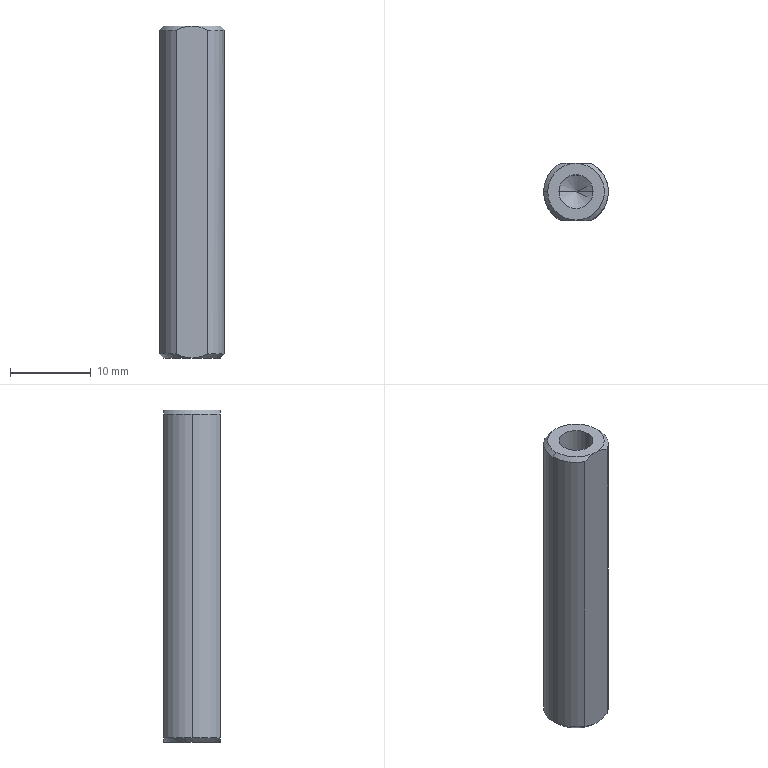Part | STEP file | 11-FG-B08411 | 1 solid | 17 faces | box 8 x 7 x 41 mm | volume 1772 mm3 | cone 8 | cylinder 5 | plane 4 | commonest cylinder face diameters 8 x3 4.2 x2
STEP:
#1=CARTESIAN_POINT('',(3.5,0.,0.));
#2=VERTEX_POINT('',#1);
#3=CARTESIAN_POINT('',(0.,-3.5,0.));
#4=VERTEX_POINT('',#3);
#5=CARTESIAN_POINT('',(0.,0.,0.));
#6=DIRECTION('',(0.,0.,-1.));
#7=DIRECTION('',(1.,0.,0.));
#8=AXIS2_PLACEMENT_3D('',#5,#6,#7);
#9=CIRCLE('',#8,3.5);
#10=EDGE_CURVE('',#2,#4,#9,.T.);
#11=ORIENTED_EDGE('',*,*,#10,.F.);
#12=CARTESIAN_POINT('',(4.,0.,0.5));
#13=VERTEX_POINT('',#12);
#14=CARTESIAN_POINT('',(4.,0.,0.5));
#15=DIRECTION('',(0.7071,0.,0.7071));
#16=VECTOR('',#15,1000.);
#17=LINE('',#14,#16);
#18=EDGE_CURVE('',#2,#13,#17,.T.);
#19=ORIENTED_EDGE('',*,*,#18,.T.);
#20=CARTESIAN_POINT('',(1.936,-3.5,0.5));
#21=VERTEX_POINT('',#20);
#22=CARTESIAN_POINT('',(0.,0.,0.5));
#23=DIRECTION('',(0.,0.,1.));
#24=DIRECTION('',(1.,0.,0.));
#25=AXIS2_PLACEMENT_3D('',#22,#23,#24);
#26=CIRCLE('',#25,4.);
#27=EDGE_CURVE('',#21,#13,#26,.T.);
#28=ORIENTED_EDGE('',*,*,#27,.F.);
#29=CARTESIAN_POINT('',(0.,-3.5,0.));
#30=CARTESIAN_POINT('',(0.3398,-3.5,0.));
#31=CARTESIAN_POINT('',(0.6708,-3.5,0.05004));
#32=CARTESIAN_POINT('',(1.157,-3.5,0.183));
#33=CARTESIAN_POINT('',(1.318,-3.5,0.2372));
#34=CARTESIAN_POINT('',(1.633,-3.5,0.3594));
#35=CARTESIAN_POINT('',(1.786,-3.5,0.4272));
#36=CARTESIAN_POINT('',(1.936,-3.5,0.5));
#37=B_SPLINE_CURVE_WITH_KNOTS('',3,(#29,#30,#31,#32,#33,#34,#35,#36),.UNSPECIFIED.,.F.,.F.,(4,2,2,4),(0.004539,0.00554,0.00604,0.006541),.UNSPECIFIED.);
#38=EDGE_CURVE('',#4,#21,#37,.T.);
#39=ORIENTED_EDGE('',*,*,#38,.F.);
#40=EDGE_LOOP('',(#11,#19,#28,#39));
#41=FACE_OUTER_BOUND('',#40,.T.);
#42=CARTESIAN_POINT('',(0.,0.,0.5));
#43=DIRECTION('',(0.,0.,1.));
#44=DIRECTION('',(1.,0.,0.));
#45=AXIS2_PLACEMENT_3D('',#42,#43,#44);
#46=CONICAL_SURFACE('',#45,4.,0.7854);
#47=ADVANCED_FACE('',(#41),#46,.T.);
#48=CARTESIAN_POINT('',(-3.5,0.,41.));
#49=VERTEX_POINT('',#48);
#50=CARTESIAN_POINT('',(0.,-3.5,41.));
#51=VERTEX_POINT('',#50);
#52=CARTESIAN_POINT('',(0.,0.,41.));
#53=DIRECTION('',(0.,0.,1.));
#54=DIRECTION('',(1.,0.,0.));
#55=AXIS2_PLACEMENT_3D('',#52,#53,#54);
#56=CIRCLE('',#55,3.5);
#57=EDGE_CURVE('',#49,#51,#56,.T.);
#58=ORIENTED_EDGE('',*,*,#57,.F.);
#59=CARTESIAN_POINT('',(-4.,0.,40.5));
#60=VERTEX_POINT('',#59);
#61=CARTESIAN_POINT('',(-3.5,0.,41.));
#62=DIRECTION('',(-0.7071,0.,-0.7071));
#63=VECTOR('',#62,1000.);
#64=LINE('',#61,#63);
#65=EDGE_CURVE('',#49,#60,#64,.T.);
#66=ORIENTED_EDGE('',*,*,#65,.T.);
#67=CARTESIAN_POINT('',(-1.936,-3.5,40.5));
#68=VERTEX_POINT('',#67);
#69=CARTESIAN_POINT('',(0.,0.,40.5));
#70=DIRECTION('',(0.,0.,-1.));
#71=DIRECTION('',(1.,0.,0.));
#72=AXIS2_PLACEMENT_3D('',#69,#70,#71);
#73=CIRCLE('',#72,4.);
#74=EDGE_CURVE('',#68,#60,#73,.T.);
#75=ORIENTED_EDGE('',*,*,#74,.F.);
#76=CARTESIAN_POINT('',(0.,-3.5,41.));
#77=CARTESIAN_POINT('',(-0.3397,-3.5,41.));
#78=CARTESIAN_POINT('',(-0.6719,-3.5,40.95));
#79=CARTESIAN_POINT('',(-1.318,-3.5,40.773));
#80=CARTESIAN_POINT('',(-1.635,-3.5,40.646));
#81=CARTESIAN_POINT('',(-1.936,-3.5,40.5));
#82=B_SPLINE_CURVE_WITH_KNOTS('',3,(#76,#77,#78,#79,#80,#81),.UNSPECIFIED.,.F.,.F.,(4,2,4),(0.004275,0.005275,0.006275),.UNSPECIFIED.);
#83=EDGE_CURVE('',#51,#68,#82,.T.);
#84=ORIENTED_EDGE('',*,*,#83,.F.);
#85=EDGE_LOOP('',(#58,#66,#75,#84));
#86=FACE_OUTER_BOUND('',#85,.T.);
#87=CARTESIAN_POINT('',(0.,0.,41.));
#88=DIRECTION('',(0.,0.,-1.));
#89=DIRECTION('',(-1.,0.,0.));
#90=AXIS2_PLACEMENT_3D('',#87,#88,#89);
#91=CONICAL_SURFACE('',#90,3.5,0.7854);
#92=ADVANCED_FACE('',(#86),#91,.T.);
#93=CARTESIAN_POINT('',(-2.1,0.,28.6));
#94=VERTEX_POINT('',#93);
#95=CARTESIAN_POINT('',(2.1,0.,28.6));
#96=VERTEX_POINT('',#95);
#97=CARTESIAN_POINT('',(0.,0.,28.6));
#98=DIRECTION('',(0.,0.,1.));
#99=DIRECTION('',(1.,0.,0.));
#100=AXIS2_PLACEMENT_3D('',#97,#98,#99);
#101=CIRCLE('',#100,2.1);
#102=EDGE_CURVE('',#94,#96,#101,.T.);
#103=ORIENTED_EDGE('',*,*,#102,.F.);
#104=CARTESIAN_POINT('',(-2.1,0.,41.));
#105=VERTEX_POINT('',#104);
#106=CARTESIAN_POINT('',(-2.1,0.,41.));
#107=DIRECTION('',(0.,0.,1.));
#108=VECTOR('',#107,1000.);
#109=LINE('',#106,#108);
#110=EDGE_CURVE('',#94,#105,#109,.T.);
#111=ORIENTED_EDGE('',*,*,#110,.T.);
#112=CARTESIAN_POINT('',(2.1,0.,41.));
#113=VERTEX_POINT('',#112);
#114=CARTESIAN_POINT('',(0.,0.,41.));
#115=DIRECTION('',(0.,0.,1.));
#116=DIRECTION('',(1.,0.,0.));
#117=AXIS2_PLACEMENT_3D('',#114,#115,#116);
#118=CIRCLE('',#117,2.1);
#119=EDGE_CURVE('',#105,#113,#118,.T.);
#120=ORIENTED_EDGE('',*,*,#119,.T.);
#121=CARTESIAN_POINT('',(2.1,0.,41.));
#122=DIRECTION('',(0.,0.,1.));
#123=VECTOR('',#122,1000.);
#124=LINE('',#121,#123);
#125=EDGE_CURVE('',#96,#113,#124,.T.);
#126=ORIENTED_EDGE('',*,*,#125,.F.);
#127=EDGE_LOOP('',(#103,#111,#120,#126));
#128=FACE_OUTER_BOUND('',#127,.T.);
#129=CARTESIAN_POINT('',(0.,0.,41.));
#130=DIRECTION('',(0.,0.,1.));
#131=DIRECTION('',(1.,0.,0.));
#132=AXIS2_PLACEMENT_3D('',#129,#130,#131);
#133=CYLINDRICAL_SURFACE('',#132,2.1);
#134=ADVANCED_FACE('',(#128),#133,.F.);
#135=CARTESIAN_POINT('',(0.,0.,27.338));
#136=VERTEX_POINT('',#135);
#137=CARTESIAN_POINT('',(2.1,0.,28.6));
#138=DIRECTION('',(0.8572,0.,0.515));
#139=VECTOR('',#138,1000.);
#140=LINE('',#137,#139);
#141=EDGE_CURVE('',#136,#96,#140,.T.);
#142=ORIENTED_EDGE('',*,*,#141,.F.);
#143=CARTESIAN_POINT('',(-2.1,0.,28.6));
#144=DIRECTION('',(-0.8572,0.,0.515));
#145=VECTOR('',#144,1000.);
#146=LINE('',#143,#145);
#147=EDGE_CURVE('',#136,#94,#146,.T.);
#148=ORIENTED_EDGE('',*,*,#147,.T.);
#149=ORIENTED_EDGE('',*,*,#102,.T.);
#150=EDGE_LOOP('',(#142,#148,#149));
#151=FACE_OUTER_BOUND('',#150,.T.);
#152=CARTESIAN_POINT('',(0.,0.,28.6));
#153=DIRECTION('',(0.,0.,1.));
#154=DIRECTION('',(1.,0.,0.));
#155=AXIS2_PLACEMENT_3D('',#152,#153,#154);
#156=CONICAL_SURFACE('',#155,2.1,1.03);
#157=ADVANCED_FACE('',(#151),#156,.F.);
#158=ORIENTED_EDGE('',*,*,#74,.T.);
#159=CARTESIAN_POINT('',(-4.,0.,0.5));
#160=VERTEX_POINT('',#159);
#161=CARTESIAN_POINT('',(-4.,0.,41.));
#162=DIRECTION('',(0.,0.,-1.));
#163=VECTOR('',#162,1000.);
#164=LINE('',#161,#163);
#165=EDGE_CURVE('',#60,#160,#164,.T.);
#166=ORIENTED_EDGE('',*,*,#165,.T.);
#167=CARTESIAN_POINT('',(-1.936,-3.5,0.5));
#168=VERTEX_POINT('',#167);
#169=CARTESIAN_POINT('',(0.,0.,0.5));
#170=DIRECTION('',(0.,0.,1.));
#171=DIRECTION('',(1.,0.,0.));
#172=AXIS2_PLACEMENT_3D('',#169,#170,#171);
#173=CIRCLE('',#172,4.);
#174=EDGE_CURVE('',#160,#168,#173,.T.);
#175=ORIENTED_EDGE('',*,*,#174,.T.);
#176=CARTESIAN_POINT('',(-1.936,-3.5,21.));
#177=DIRECTION('',(0.,0.,1.));
#178=VECTOR('',#177,1000.);
#179=LINE('',#176,#178);
#180=EDGE_CURVE('',#168,#68,#179,.T.);
#181=ORIENTED_EDGE('',*,*,#180,.T.);
#182=EDGE_LOOP('',(#158,#166,#175,#181));
#183=FACE_OUTER_BOUND('',#182,.T.);
#184=CARTESIAN_POINT('',(0.,0.,41.));
#185=DIRECTION('',(0.,0.,-1.));
#186=DIRECTION('',(-1.,0.,0.));
#187=AXIS2_PLACEMENT_3D('',#184,#185,#186);
#188=CYLINDRICAL_SURFACE('',#187,4.);
#189=ADVANCED_FACE('',(#183),#188,.T.);
#190=CARTESIAN_POINT('',(1.936,3.5,40.5));
#191=VERTEX_POINT('',#190);
#192=CARTESIAN_POINT('',(1.936,-3.5,40.5));
#193=VERTEX_POINT('',#192);
#194=CARTESIAN_POINT('',(0.,0.,40.5));
#195=DIRECTION('',(0.,0.,-1.));
#196=DIRECTION('',(1.,0.,0.));
#197=AXIS2_PLACEMENT_3D('',#194,#195,#196);
#198=CIRCLE('',#197,4.);
#199=EDGE_CURVE('',#191,#193,#198,.T.);
#200=ORIENTED_EDGE('',*,*,#199,.T.);
#201=CARTESIAN_POINT('',(1.936,-3.5,21.));
#202=DIRECTION('',(0.,0.,1.));
#203=VECTOR('',#202,1000.);
#204=LINE('',#201,#203);
#205=EDGE_CURVE('',#21,#193,#204,.T.);
#206=ORIENTED_EDGE('',*,*,#205,.F.);
#207=ORIENTED_EDGE('',*,*,#27,.T.);
#208=CARTESIAN_POINT('',(1.936,3.5,0.5));
#209=VERTEX_POINT('',#208);
#210=CARTESIAN_POINT('',(0.,0.,0.5));
#211=DIRECTION('',(0.,0.,1.));
#212=DIRECTION('',(1.,0.,0.));
#213=AXIS2_PLACEMENT_3D('',#210,#211,#212);
#214=CIRCLE('',#213,4.);
#215=EDGE_CURVE('',#13,#209,#214,.T.);
#216=ORIENTED_EDGE('',*,*,#215,.T.);
#217=CARTESIAN_POINT('',(1.936,3.5,21.));
#218=DIRECTION('',(0.,0.,1.));
#219=VECTOR('',#218,1000.);
#220=LINE('',#217,#219);
#221=EDGE_CURVE('',#209,#191,#220,.T.);
#222=ORIENTED_EDGE('',*,*,#221,.T.);
#223=EDGE_LOOP('',(#200,#206,#207,#216,#222));
#224=FACE_OUTER_BOUND('',#223,.T.);
#225=CARTESIAN_POINT('',(0.,0.,41.));
#226=DIRECTION('',(0.,0.,-1.));
#227=DIRECTION('',(-1.,0.,0.));
#228=AXIS2_PLACEMENT_3D('',#225,#226,#227);
#229=CYLINDRICAL_SURFACE('',#228,4.);
#230=ADVANCED_FACE('',(#224),#229,.T.);
#231=CARTESIAN_POINT('',(1.936,-3.5,40.5));
#232=CARTESIAN_POINT('',(1.786,-3.5,40.573));
#233=CARTESIAN_POINT('',(1.633,-3.5,40.641));
#234=CARTESIAN_POINT('',(1.318,-3.5,40.763));
#235=CARTESIAN_POINT('',(1.157,-3.5,40.817));
#236=CARTESIAN_POINT('',(0.6708,-3.5,40.95));
#237=CARTESIAN_POINT('',(0.3398,-3.5,41.));
#238=CARTESIAN_POINT('',(0.,-3.5,41.));
#239=B_SPLINE_CURVE_WITH_KNOTS('',3,(#231,#232,#233,#234,#235,#236,#237,#238),.UNSPECIFIED.,.F.,.F.,(4,2,2,4),(0.002275,0.002775,0.003275,0.004275),.UNSPECIFIED.);
#240=EDGE_CURVE('',#193,#51,#239,.T.);
#241=ORIENTED_EDGE('',*,*,#240,.F.);
#242=ORIENTED_EDGE('',*,*,#199,.F.);
#243=CARTESIAN_POINT('',(0.,3.5,41.));
#244=VERTEX_POINT('',#243);
#245=CARTESIAN_POINT('',(0.,3.5,41.));
#246=CARTESIAN_POINT('',(0.3398,3.5,41.));
#247=CARTESIAN_POINT('',(0.6708,3.5,40.95));
#248=CARTESIAN_POINT('',(1.157,3.5,40.817));
#249=CARTESIAN_POINT('',(1.318,3.5,40.763));
#250=CARTESIAN_POINT('',(1.633,3.5,40.641));
#251=CARTESIAN_POINT('',(1.786,3.5,40.573));
#252=CARTESIAN_POINT('',(1.936,3.5,40.5));
#253=B_SPLINE_CURVE_WITH_KNOTS('',3,(#245,#246,#247,#248,#249,#250,#251,#252),.UNSPECIFIED.,.F.,.F.,(4,2,2,4),(0.004539,0.00554,0.00604,0.006541),.UNSPECIFIED.);
#254=EDGE_CURVE('',#244,#191,#253,.T.);
#255=ORIENTED_EDGE('',*,*,#254,.F.);
#256=CARTESIAN_POINT('',(0.,0.,41.));
#257=DIRECTION('',(0.,0.,1.));
#258=DIRECTION('',(1.,0.,0.));
#259=AXIS2_PLACEMENT_3D('',#256,#257,#258);
#260=CIRCLE('',#259,3.5);
#261=EDGE_CURVE('',#51,#244,#260,.T.);
#262=ORIENTED_EDGE('',*,*,#261,.F.);
#263=EDGE_LOOP('',(#241,#242,#255,#262));
#264=FACE_OUTER_BOUND('',#263,.T.);
#265=CARTESIAN_POINT('',(0.,0.,41.));
#266=DIRECTION('',(0.,0.,-1.));
#267=DIRECTION('',(-1.,0.,0.));
#268=AXIS2_PLACEMENT_3D('',#265,#266,#267);
#269=CONICAL_SURFACE('',#268,3.5,0.7854);
#270=ADVANCED_FACE('',(#264),#269,.T.);
#271=CARTESIAN_POINT('',(-1.936,-3.5,0.5));
#272=CARTESIAN_POINT('',(-1.635,-3.5,0.3541));
#273=CARTESIAN_POINT('',(-1.318,-3.5,0.2271));
#274=CARTESIAN_POINT('',(-0.6719,-3.5,0.05033));
#275=CARTESIAN_POINT('',(-0.3397,-3.5,0.));
#276=CARTESIAN_POINT('',(0.,-3.5,0.));
#277=B_SPLINE_CURVE_WITH_KNOTS('',3,(#271,#272,#273,#274,#275,#276),.UNSPECIFIED.,.F.,.F.,(4,2,4),(0.002539,0.003539,0.004539),.UNSPECIFIED.);
#278=EDGE_CURVE('',#168,#4,#277,.T.);
#279=ORIENTED_EDGE('',*,*,#278,.F.);
#280=ORIENTED_EDGE('',*,*,#174,.F.);
#281=CARTESIAN_POINT('',(-1.936,3.5,0.5));
#282=VERTEX_POINT('',#281);
#283=CARTESIAN_POINT('',(0.,0.,0.5));
#284=DIRECTION('',(0.,0.,1.));
#285=DIRECTION('',(1.,0.,0.));
#286=AXIS2_PLACEMENT_3D('',#283,#284,#285);
#287=CIRCLE('',#286,4.);
#288=EDGE_CURVE('',#282,#160,#287,.T.);
#289=ORIENTED_EDGE('',*,*,#288,.F.);
#290=CARTESIAN_POINT('',(0.,3.5,0.));
#291=VERTEX_POINT('',#290);
#292=CARTESIAN_POINT('',(0.,3.5,0.));
#293=CARTESIAN_POINT('',(-0.3397,3.5,0.));
#294=CARTESIAN_POINT('',(-0.6719,3.5,0.05033));
#295=CARTESIAN_POINT('',(-1.318,3.5,0.2271));
#296=CARTESIAN_POINT('',(-1.635,3.5,0.3541));
#297=CARTESIAN_POINT('',(-1.936,3.5,0.5));
#298=B_SPLINE_CURVE_WITH_KNOTS('',3,(#292,#293,#294,#295,#296,#297),.UNSPECIFIED.,.F.,.F.,(4,2,4),(0.004275,0.005275,0.006275),.UNSPECIFIED.);
#299=EDGE_CURVE('',#291,#282,#298,.T.);
#300=ORIENTED_EDGE('',*,*,#299,.F.);
#301=CARTESIAN_POINT('',(0.,0.,0.));
#302=DIRECTION('',(0.,0.,-1.));
#303=DIRECTION('',(1.,0.,0.));
#304=AXIS2_PLACEMENT_3D('',#301,#302,#303);
#305=CIRCLE('',#304,3.5);
#306=EDGE_CURVE('',#4,#291,#305,.T.);
#307=ORIENTED_EDGE('',*,*,#306,.F.);
#308=EDGE_LOOP('',(#279,#280,#289,#300,#307));
#309=FACE_OUTER_BOUND('',#308,.T.);
#310=CARTESIAN_POINT('',(0.,0.,0.5));
#311=DIRECTION('',(0.,0.,1.));
#312=DIRECTION('',(1.,0.,0.));
#313=AXIS2_PLACEMENT_3D('',#310,#311,#312);
#314=CONICAL_SURFACE('',#313,4.,0.7854);
#315=ADVANCED_FACE('',(#309),#314,.T.);
#316=ORIENTED_EDGE('',*,*,#165,.F.);
#317=CARTESIAN_POINT('',(-1.936,3.5,40.5));
#318=VERTEX_POINT('',#317);
#319=CARTESIAN_POINT('',(0.,0.,40.5));
#320=DIRECTION('',(0.,0.,-1.));
#321=DIRECTION('',(1.,0.,0.));
#322=AXIS2_PLACEMENT_3D('',#319,#320,#321);
#323=CIRCLE('',#322,4.);
#324=EDGE_CURVE('',#60,#318,#323,.T.);
#325=ORIENTED_EDGE('',*,*,#324,.T.);
#326=CARTESIAN_POINT('',(-1.936,3.5,21.));
#327=DIRECTION('',(0.,0.,1.));
#328=VECTOR('',#327,1000.);
#329=LINE('',#326,#328);
#330=EDGE_CURVE('',#282,#318,#329,.T.);
#331=ORIENTED_EDGE('',*,*,#330,.F.);
#332=ORIENTED_EDGE('',*,*,#288,.T.);
#333=EDGE_LOOP('',(#316,#325,#331,#332));
#334=FACE_OUTER_BOUND('',#333,.T.);
#335=CARTESIAN_POINT('',(0.,0.,41.));
#336=DIRECTION('',(0.,0.,-1.));
#337=DIRECTION('',(-1.,0.,0.));
#338=AXIS2_PLACEMENT_3D('',#335,#336,#337);
#339=CYLINDRICAL_SURFACE('',#338,4.);
#340=ADVANCED_FACE('',(#334),#339,.T.);
#341=CARTESIAN_POINT('',(0.,0.,41.));
#342=DIRECTION('',(0.,0.,1.));
#343=DIRECTION('',(1.,0.,0.));
#344=AXIS2_PLACEMENT_3D('',#341,#342,#343);
#345=CIRCLE('',#344,3.5);
#346=EDGE_CURVE('',#244,#49,#345,.T.);
#347=ORIENTED_EDGE('',*,*,#346,.T.);
#348=ORIENTED_EDGE('',*,*,#57,.T.);
#349=ORIENTED_EDGE('',*,*,#261,.T.);
#350=EDGE_LOOP('',(#347,#348,#349));
#351=FACE_OUTER_BOUND('',#350,.T.);
#352=CARTESIAN_POINT('',(0.,0.,41.));
#353=DIRECTION('',(0.,0.,1.));
#354=DIRECTION('',(1.,0.,0.));
#355=AXIS2_PLACEMENT_3D('',#352,#353,#354);
#356=CIRCLE('',#355,2.1);
#357=EDGE_CURVE('',#113,#105,#356,.T.);
#358=ORIENTED_EDGE('',*,*,#357,.F.);
#359=ORIENTED_EDGE('',*,*,#119,.F.);
#360=EDGE_LOOP('',(#358,#359));
#361=FACE_BOUND('',#360,.T.);
#362=CARTESIAN_POINT('',(0.,0.,41.));
#363=DIRECTION('',(0.,0.,1.));
#364=DIRECTION('',(1.,0.,0.));
#365=AXIS2_PLACEMENT_3D('',#362,#363,#364);
#366=PLANE('',#365);
#367=ADVANCED_FACE('',(#351,#361),#366,.T.);
#368=CARTESIAN_POINT('',(0.,0.,0.));
#369=DIRECTION('',(0.,0.,-1.));
#370=DIRECTION('',(1.,0.,0.));
#371=AXIS2_PLACEMENT_3D('',#368,#369,#370);
#372=CIRCLE('',#371,3.5);
#373=EDGE_CURVE('',#291,#2,#372,.T.);
#374=ORIENTED_EDGE('',*,*,#373,.T.);
#375=ORIENTED_EDGE('',*,*,#10,.T.);
#376=ORIENTED_EDGE('',*,*,#306,.T.);
#377=EDGE_LOOP('',(#374,#375,#376));
#378=FACE_OUTER_BOUND('',#377,.T.);
#379=CARTESIAN_POINT('',(0.,0.,0.));
#380=DIRECTION('',(0.,0.,1.));
#381=DIRECTION('',(1.,0.,0.));
#382=AXIS2_PLACEMENT_3D('',#379,#380,#381);
#383=PLANE('',#382);
#384=ADVANCED_FACE('',(#378),#383,.F.);
#385=ORIENTED_EDGE('',*,*,#147,.F.);
#386=ORIENTED_EDGE('',*,*,#141,.T.);
#387=CARTESIAN_POINT('',(0.,0.,28.6));
#388=DIRECTION('',(0.,0.,1.));
#389=DIRECTION('',(1.,0.,0.));
#390=AXIS2_PLACEMENT_3D('',#387,#388,#389);
#391=CIRCLE('',#390,2.1);
#392=EDGE_CURVE('',#96,#94,#391,.T.);
#393=ORIENTED_EDGE('',*,*,#392,.T.);
#394=EDGE_LOOP('',(#385,#386,#393));
#395=FACE_OUTER_BOUND('',#394,.T.);
#396=CARTESIAN_POINT('',(0.,0.,28.6));
#397=DIRECTION('',(0.,0.,1.));
#398=DIRECTION('',(1.,0.,0.));
#399=AXIS2_PLACEMENT_3D('',#396,#397,#398);
#400=CONICAL_SURFACE('',#399,2.1,1.03);
#401=ADVANCED_FACE('',(#395),#400,.F.);
#402=ORIENTED_EDGE('',*,*,#110,.F.);
#403=ORIENTED_EDGE('',*,*,#392,.F.);
#404=ORIENTED_EDGE('',*,*,#125,.T.);
#405=ORIENTED_EDGE('',*,*,#357,.T.);
#406=EDGE_LOOP('',(#402,#403,#404,#405));
#407=FACE_OUTER_BOUND('',#406,.T.);
#408=CARTESIAN_POINT('',(0.,0.,41.));
#409=DIRECTION('',(0.,0.,1.));
#410=DIRECTION('',(1.,0.,0.));
#411=AXIS2_PLACEMENT_3D('',#408,#409,#410);
#412=CYLINDRICAL_SURFACE('',#411,2.1);
#413=ADVANCED_FACE('',(#407),#412,.F.);
#414=ORIENTED_EDGE('',*,*,#65,.F.);
#415=ORIENTED_EDGE('',*,*,#346,.F.);
#416=CARTESIAN_POINT('',(-1.936,3.5,40.5));
#417=CARTESIAN_POINT('',(-1.635,3.5,40.646));
#418=CARTESIAN_POINT('',(-1.318,3.5,40.773));
#419=CARTESIAN_POINT('',(-0.6719,3.5,40.95));
#420=CARTESIAN_POINT('',(-0.3397,3.5,41.));
#421=CARTESIAN_POINT('',(0.,3.5,41.));
#422=B_SPLINE_CURVE_WITH_KNOTS('',3,(#416,#417,#418,#419,#420,#421),.UNSPECIFIED.,.F.,.F.,(4,2,4),(0.002539,0.003539,0.004539),.UNSPECIFIED.);
#423=EDGE_CURVE('',#318,#244,#422,.T.);
#424=ORIENTED_EDGE('',*,*,#423,.F.);
#425=ORIENTED_EDGE('',*,*,#324,.F.);
#426=EDGE_LOOP('',(#414,#415,#424,#425));
#427=FACE_OUTER_BOUND('',#426,.T.);
#428=CARTESIAN_POINT('',(0.,0.,41.));
#429=DIRECTION('',(0.,0.,-1.));
#430=DIRECTION('',(-1.,0.,0.));
#431=AXIS2_PLACEMENT_3D('',#428,#429,#430);
#432=CONICAL_SURFACE('',#431,3.5,0.7854);
#433=ADVANCED_FACE('',(#427),#432,.T.);
#434=ORIENTED_EDGE('',*,*,#18,.F.);
#435=ORIENTED_EDGE('',*,*,#373,.F.);
#436=CARTESIAN_POINT('',(1.936,3.5,0.5));
#437=CARTESIAN_POINT('',(1.786,3.5,0.4272));
#438=CARTESIAN_POINT('',(1.633,3.5,0.3594));
#439=CARTESIAN_POINT('',(1.318,3.5,0.2372));
#440=CARTESIAN_POINT('',(1.157,3.5,0.183));
#441=CARTESIAN_POINT('',(0.6708,3.5,0.05004));
#442=CARTESIAN_POINT('',(0.3398,3.5,0.));
#443=CARTESIAN_POINT('',(0.,3.5,0.));
#444=B_SPLINE_CURVE_WITH_KNOTS('',3,(#436,#437,#438,#439,#440,#441,#442,#443),.UNSPECIFIED.,.F.,.F.,(4,2,2,4),(0.002275,0.002775,0.003275,0.004275),.UNSPECIFIED.);
#445=EDGE_CURVE('',#209,#291,#444,.T.);
#446=ORIENTED_EDGE('',*,*,#445,.F.);
#447=ORIENTED_EDGE('',*,*,#215,.F.);
#448=EDGE_LOOP('',(#434,#435,#446,#447));
#449=FACE_OUTER_BOUND('',#448,.T.);
#450=CARTESIAN_POINT('',(0.,0.,0.5));
#451=DIRECTION('',(0.,0.,1.));
#452=DIRECTION('',(1.,0.,0.));
#453=AXIS2_PLACEMENT_3D('',#450,#451,#452);
#454=CONICAL_SURFACE('',#453,4.,0.7854);
#455=ADVANCED_FACE('',(#449),#454,.T.);
#456=ORIENTED_EDGE('',*,*,#330,.T.);
#457=ORIENTED_EDGE('',*,*,#423,.T.);
#458=ORIENTED_EDGE('',*,*,#254,.T.);
#459=ORIENTED_EDGE('',*,*,#221,.F.);
#460=ORIENTED_EDGE('',*,*,#445,.T.);
#461=ORIENTED_EDGE('',*,*,#299,.T.);
#462=EDGE_LOOP('',(#456,#457,#458,#459,#460,#461));
#463=FACE_OUTER_BOUND('',#462,.T.);
#464=CARTESIAN_POINT('',(-1.936,3.5,21.));
#465=DIRECTION('',(0.,-1.,0.));
#466=DIRECTION('',(0.,0.,-1.));
#467=AXIS2_PLACEMENT_3D('',#464,#465,#466);
#468=PLANE('',#467);
#469=ADVANCED_FACE('',(#463),#468,.F.);
#470=ORIENTED_EDGE('',*,*,#205,.T.);
#471=ORIENTED_EDGE('',*,*,#240,.T.);
#472=ORIENTED_EDGE('',*,*,#83,.T.);
#473=ORIENTED_EDGE('',*,*,#180,.F.);
#474=ORIENTED_EDGE('',*,*,#278,.T.);
#475=ORIENTED_EDGE('',*,*,#38,.T.);
#476=EDGE_LOOP('',(#470,#471,#472,#473,#474,#475));
#477=FACE_OUTER_BOUND('',#476,.T.);
#478=CARTESIAN_POINT('',(-1.936,-3.5,21.));
#479=DIRECTION('',(0.,1.,0.));
#480=DIRECTION('',(0.,0.,1.));
#481=AXIS2_PLACEMENT_3D('',#478,#479,#480);
#482=PLANE('',#481);
#483=ADVANCED_FACE('',(#477),#482,.F.);
#484=CLOSED_SHELL('',(#47,#92,#134,#157,#189,#230,#270,#315,#340,#367,#384,#401,#413,#433,#455,#469,#483));
#485=MANIFOLD_SOLID_BREP('',#484);
#486=CARTESIAN_POINT('',(0.,0.,0.));
#487=DIRECTION('',(0.,0.,1.));
#488=DIRECTION('',(1.,0.,0.));
#489=AXIS2_PLACEMENT_3D('',#486,#487,#488);
#490=(LENGTH_UNIT()NAMED_UNIT(*)SI_UNIT(.MILLI.,.METRE.));
#491=UNCERTAINTY_MEASURE_WITH_UNIT(LENGTH_MEASURE(0.00001),#490,'','');
#492=(NAMED_UNIT(*)PLANE_ANGLE_UNIT()SI_UNIT($,.RADIAN.));
#493=(NAMED_UNIT(*)SI_UNIT($,.STERADIAN.)SOLID_ANGLE_UNIT());
#494=(GEOMETRIC_REPRESENTATION_CONTEXT(3)GLOBAL_UNCERTAINTY_ASSIGNED_CONTEXT((#491))GLOBAL_UNIT_ASSIGNED_CONTEXT((#490,#492,#493))REPRESENTATION_CONTEXT('',''));
#495=ADVANCED_BREP_SHAPE_REPRESENTATION('',(#485,#489),#494);